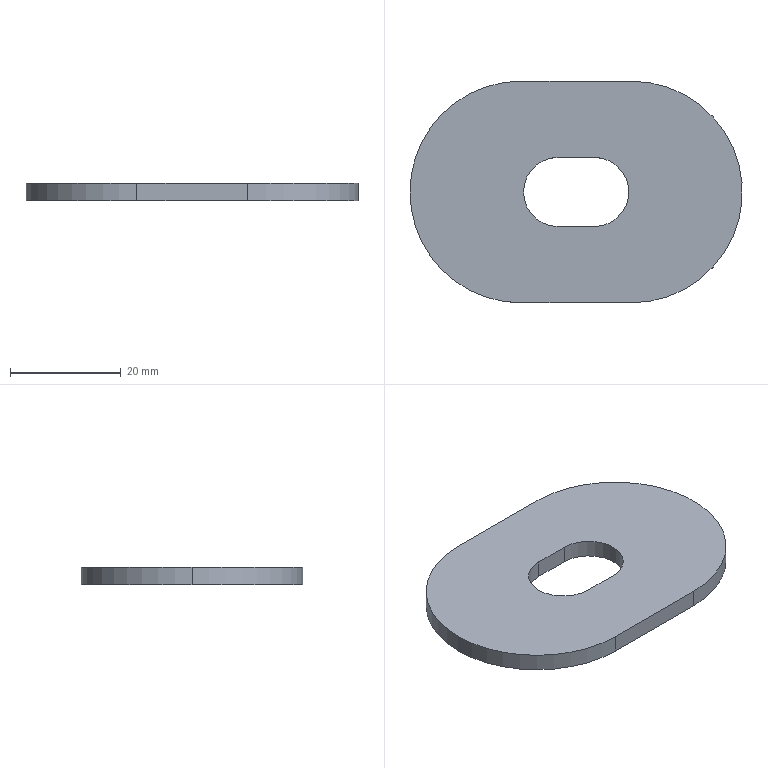Part | SolidWorks | features FlatPattern 1, SMBaseFlange 1, SheetMetal 1 | 1 solid | 12 faces | box 60 x 40 x 3.2 mm | volume 5929 mm3 | cylinder 6 | plane 6 | commonest cylinder face diameters 12.5 x3 40 x3
STEP:
#1=CARTESIAN_POINT('',(575.75,726.25,3.2));
#2=VERTEX_POINT('',#1);
#3=CARTESIAN_POINT('',(569.5,720.,3.2));
#4=VERTEX_POINT('',#3);
#5=CARTESIAN_POINT('',(575.75,720.,3.2));
#6=DIRECTION('',(0.,0.,1.));
#7=DIRECTION('',(1.,0.,0.));
#8=AXIS2_PLACEMENT_3D('',#5,#6,#7);
#9=CIRCLE('',#8,6.25);
#10=EDGE_CURVE('',#2,#4,#9,.T.);
#11=ORIENTED_EDGE('',*,*,#10,.T.);
#12=CARTESIAN_POINT('',(569.5,720.,0.));
#13=VERTEX_POINT('',#12);
#14=CARTESIAN_POINT('',(569.5,720.,3.2));
#15=DIRECTION('',(0.,0.,-1.));
#16=VECTOR('',#15,1000.);
#17=LINE('',#14,#16);
#18=EDGE_CURVE('',#4,#13,#17,.T.);
#19=ORIENTED_EDGE('',*,*,#18,.T.);
#20=CARTESIAN_POINT('',(575.75,726.25,0.));
#21=VERTEX_POINT('',#20);
#22=CARTESIAN_POINT('',(575.75,720.,0.));
#23=DIRECTION('',(0.,0.,1.));
#24=DIRECTION('',(1.,0.,0.));
#25=AXIS2_PLACEMENT_3D('',#22,#23,#24);
#26=CIRCLE('',#25,6.25);
#27=EDGE_CURVE('',#21,#13,#26,.T.);
#28=ORIENTED_EDGE('',*,*,#27,.F.);
#29=CARTESIAN_POINT('',(575.75,726.25,3.2));
#30=DIRECTION('',(0.,0.,-1.));
#31=VECTOR('',#30,1000.);
#32=LINE('',#29,#31);
#33=EDGE_CURVE('',#2,#21,#32,.T.);
#34=ORIENTED_EDGE('',*,*,#33,.F.);
#35=EDGE_LOOP('',(#11,#19,#28,#34));
#36=FACE_OUTER_BOUND('',#35,.T.);
#37=CARTESIAN_POINT('',(575.75,720.,3.2));
#38=DIRECTION('',(0.,0.,-1.));
#39=DIRECTION('',(-1.,0.,0.));
#40=AXIS2_PLACEMENT_3D('',#37,#38,#39);
#41=CYLINDRICAL_SURFACE('',#40,6.25);
#42=ADVANCED_FACE('',(#36),#41,.F.);
#43=CARTESIAN_POINT('',(549.,720.,3.2));
#44=VERTEX_POINT('',#43);
#45=CARTESIAN_POINT('',(569.,700.,3.2));
#46=VERTEX_POINT('',#45);
#47=CARTESIAN_POINT('',(569.,720.,3.2));
#48=DIRECTION('',(0.,0.,1.));
#49=DIRECTION('',(1.,0.,0.));
#50=AXIS2_PLACEMENT_3D('',#47,#48,#49);
#51=CIRCLE('',#50,20.);
#52=EDGE_CURVE('',#44,#46,#51,.T.);
#53=ORIENTED_EDGE('',*,*,#52,.F.);
#54=CARTESIAN_POINT('',(549.,720.,0.));
#55=VERTEX_POINT('',#54);
#56=CARTESIAN_POINT('',(549.,720.,3.2));
#57=DIRECTION('',(0.,0.,-1.));
#58=VECTOR('',#57,1000.);
#59=LINE('',#56,#58);
#60=EDGE_CURVE('',#44,#55,#59,.T.);
#61=ORIENTED_EDGE('',*,*,#60,.T.);
#62=CARTESIAN_POINT('',(569.,700.,0.));
#63=VERTEX_POINT('',#62);
#64=CARTESIAN_POINT('',(569.,720.,0.));
#65=DIRECTION('',(0.,0.,1.));
#66=DIRECTION('',(1.,0.,0.));
#67=AXIS2_PLACEMENT_3D('',#64,#65,#66);
#68=CIRCLE('',#67,20.);
#69=EDGE_CURVE('',#55,#63,#68,.T.);
#70=ORIENTED_EDGE('',*,*,#69,.T.);
#71=CARTESIAN_POINT('',(569.,700.,3.2));
#72=DIRECTION('',(0.,0.,-1.));
#73=VECTOR('',#72,1000.);
#74=LINE('',#71,#73);
#75=EDGE_CURVE('',#46,#63,#74,.T.);
#76=ORIENTED_EDGE('',*,*,#75,.F.);
#77=EDGE_LOOP('',(#53,#61,#70,#76));
#78=FACE_OUTER_BOUND('',#77,.T.);
#79=CARTESIAN_POINT('',(569.,720.,3.2));
#80=DIRECTION('',(0.,0.,-1.));
#81=DIRECTION('',(-1.,0.,0.));
#82=AXIS2_PLACEMENT_3D('',#79,#80,#81);
#83=CYLINDRICAL_SURFACE('',#82,20.);
#84=ADVANCED_FACE('',(#78),#83,.T.);
#85=CARTESIAN_POINT('',(569.,740.,3.2));
#86=VERTEX_POINT('',#85);
#87=CARTESIAN_POINT('',(569.,720.,3.2));
#88=DIRECTION('',(0.,0.,1.));
#89=DIRECTION('',(1.,0.,0.));
#90=AXIS2_PLACEMENT_3D('',#87,#88,#89);
#91=CIRCLE('',#90,20.);
#92=EDGE_CURVE('',#86,#44,#91,.T.);
#93=ORIENTED_EDGE('',*,*,#92,.T.);
#94=ORIENTED_EDGE('',*,*,#52,.T.);
#95=CARTESIAN_POINT('',(589.,700.,3.2));
#96=VERTEX_POINT('',#95);
#97=CARTESIAN_POINT('',(569.,700.,3.2));
#98=DIRECTION('',(1.,0.,0.));
#99=VECTOR('',#98,1000.);
#100=LINE('',#97,#99);
#101=EDGE_CURVE('',#46,#96,#100,.T.);
#102=ORIENTED_EDGE('',*,*,#101,.T.);
#103=CARTESIAN_POINT('',(589.,740.,3.2));
#104=VERTEX_POINT('',#103);
#105=CARTESIAN_POINT('',(589.,720.,3.2));
#106=DIRECTION('',(0.,0.,1.));
#107=DIRECTION('',(1.,0.,0.));
#108=AXIS2_PLACEMENT_3D('',#105,#106,#107);
#109=CIRCLE('',#108,20.);
#110=EDGE_CURVE('',#96,#104,#109,.T.);
#111=ORIENTED_EDGE('',*,*,#110,.T.);
#112=CARTESIAN_POINT('',(569.,740.,3.2));
#113=DIRECTION('',(-1.,0.,0.));
#114=VECTOR('',#113,1000.);
#115=LINE('',#112,#114);
#116=EDGE_CURVE('',#104,#86,#115,.T.);
#117=ORIENTED_EDGE('',*,*,#116,.T.);
#118=EDGE_LOOP('',(#93,#94,#102,#111,#117));
#119=FACE_OUTER_BOUND('',#118,.T.);
#120=CARTESIAN_POINT('',(575.75,713.75,3.2));
#121=VERTEX_POINT('',#120);
#122=CARTESIAN_POINT('',(582.25,713.75,3.2));
#123=VERTEX_POINT('',#122);
#124=CARTESIAN_POINT('',(575.75,713.75,3.2));
#125=DIRECTION('',(1.,0.,0.));
#126=VECTOR('',#125,1000.);
#127=LINE('',#124,#126);
#128=EDGE_CURVE('',#121,#123,#127,.T.);
#129=ORIENTED_EDGE('',*,*,#128,.F.);
#130=CARTESIAN_POINT('',(575.75,720.,3.2));
#131=DIRECTION('',(0.,0.,1.));
#132=DIRECTION('',(1.,0.,0.));
#133=AXIS2_PLACEMENT_3D('',#130,#131,#132);
#134=CIRCLE('',#133,6.25);
#135=EDGE_CURVE('',#4,#121,#134,.T.);
#136=ORIENTED_EDGE('',*,*,#135,.F.);
#137=ORIENTED_EDGE('',*,*,#10,.F.);
#138=CARTESIAN_POINT('',(582.25,726.25,3.2));
#139=VERTEX_POINT('',#138);
#140=CARTESIAN_POINT('',(575.75,726.25,3.2));
#141=DIRECTION('',(-1.,0.,0.));
#142=VECTOR('',#141,1000.);
#143=LINE('',#140,#142);
#144=EDGE_CURVE('',#139,#2,#143,.T.);
#145=ORIENTED_EDGE('',*,*,#144,.F.);
#146=CARTESIAN_POINT('',(582.25,720.,3.2));
#147=DIRECTION('',(0.,0.,1.));
#148=DIRECTION('',(1.,0.,0.));
#149=AXIS2_PLACEMENT_3D('',#146,#147,#148);
#150=CIRCLE('',#149,6.25);
#151=EDGE_CURVE('',#123,#139,#150,.T.);
#152=ORIENTED_EDGE('',*,*,#151,.F.);
#153=EDGE_LOOP('',(#129,#136,#137,#145,#152));
#154=FACE_BOUND('',#153,.T.);
#155=CARTESIAN_POINT('',(569.,720.,3.2));
#156=DIRECTION('',(0.,0.,1.));
#157=DIRECTION('',(1.,0.,0.));
#158=AXIS2_PLACEMENT_3D('',#155,#156,#157);
#159=PLANE('',#158);
#160=ADVANCED_FACE('',(#119,#154),#159,.T.);
#161=CARTESIAN_POINT('',(569.,740.,0.));
#162=VERTEX_POINT('',#161);
#163=CARTESIAN_POINT('',(569.,720.,0.));
#164=DIRECTION('',(0.,0.,1.));
#165=DIRECTION('',(1.,0.,0.));
#166=AXIS2_PLACEMENT_3D('',#163,#164,#165);
#167=CIRCLE('',#166,20.);
#168=EDGE_CURVE('',#162,#55,#167,.T.);
#169=ORIENTED_EDGE('',*,*,#168,.F.);
#170=CARTESIAN_POINT('',(589.,740.,0.));
#171=VERTEX_POINT('',#170);
#172=CARTESIAN_POINT('',(569.,740.,0.));
#173=DIRECTION('',(-1.,0.,0.));
#174=VECTOR('',#173,1000.);
#175=LINE('',#172,#174);
#176=EDGE_CURVE('',#171,#162,#175,.T.);
#177=ORIENTED_EDGE('',*,*,#176,.F.);
#178=CARTESIAN_POINT('',(589.,700.,0.));
#179=VERTEX_POINT('',#178);
#180=CARTESIAN_POINT('',(589.,720.,0.));
#181=DIRECTION('',(0.,0.,1.));
#182=DIRECTION('',(1.,0.,0.));
#183=AXIS2_PLACEMENT_3D('',#180,#181,#182);
#184=CIRCLE('',#183,20.);
#185=EDGE_CURVE('',#179,#171,#184,.T.);
#186=ORIENTED_EDGE('',*,*,#185,.F.);
#187=CARTESIAN_POINT('',(569.,700.,0.));
#188=DIRECTION('',(1.,0.,0.));
#189=VECTOR('',#188,1000.);
#190=LINE('',#187,#189);
#191=EDGE_CURVE('',#63,#179,#190,.T.);
#192=ORIENTED_EDGE('',*,*,#191,.F.);
#193=ORIENTED_EDGE('',*,*,#69,.F.);
#194=EDGE_LOOP('',(#169,#177,#186,#192,#193));
#195=FACE_OUTER_BOUND('',#194,.T.);
#196=ORIENTED_EDGE('',*,*,#27,.T.);
#197=CARTESIAN_POINT('',(575.75,713.75,0.));
#198=VERTEX_POINT('',#197);
#199=CARTESIAN_POINT('',(575.75,720.,0.));
#200=DIRECTION('',(0.,0.,1.));
#201=DIRECTION('',(1.,0.,0.));
#202=AXIS2_PLACEMENT_3D('',#199,#200,#201);
#203=CIRCLE('',#202,6.25);
#204=EDGE_CURVE('',#13,#198,#203,.T.);
#205=ORIENTED_EDGE('',*,*,#204,.T.);
#206=CARTESIAN_POINT('',(582.25,713.75,0.));
#207=VERTEX_POINT('',#206);
#208=CARTESIAN_POINT('',(575.75,713.75,0.));
#209=DIRECTION('',(1.,0.,0.));
#210=VECTOR('',#209,1000.);
#211=LINE('',#208,#210);
#212=EDGE_CURVE('',#198,#207,#211,.T.);
#213=ORIENTED_EDGE('',*,*,#212,.T.);
#214=CARTESIAN_POINT('',(582.25,726.25,0.));
#215=VERTEX_POINT('',#214);
#216=CARTESIAN_POINT('',(582.25,720.,0.));
#217=DIRECTION('',(0.,0.,1.));
#218=DIRECTION('',(1.,0.,0.));
#219=AXIS2_PLACEMENT_3D('',#216,#217,#218);
#220=CIRCLE('',#219,6.25);
#221=EDGE_CURVE('',#207,#215,#220,.T.);
#222=ORIENTED_EDGE('',*,*,#221,.T.);
#223=CARTESIAN_POINT('',(575.75,726.25,0.));
#224=DIRECTION('',(-1.,0.,0.));
#225=VECTOR('',#224,1000.);
#226=LINE('',#223,#225);
#227=EDGE_CURVE('',#215,#21,#226,.T.);
#228=ORIENTED_EDGE('',*,*,#227,.T.);
#229=EDGE_LOOP('',(#196,#205,#213,#222,#228));
#230=FACE_BOUND('',#229,.T.);
#231=CARTESIAN_POINT('',(569.,720.,0.));
#232=DIRECTION('',(0.,0.,1.));
#233=DIRECTION('',(1.,0.,0.));
#234=AXIS2_PLACEMENT_3D('',#231,#232,#233);
#235=PLANE('',#234);
#236=ADVANCED_FACE('',(#195,#230),#235,.F.);
#237=ORIENTED_EDGE('',*,*,#60,.F.);
#238=ORIENTED_EDGE('',*,*,#92,.F.);
#239=CARTESIAN_POINT('',(569.,740.,3.2));
#240=DIRECTION('',(0.,0.,-1.));
#241=VECTOR('',#240,1000.);
#242=LINE('',#239,#241);
#243=EDGE_CURVE('',#86,#162,#242,.T.);
#244=ORIENTED_EDGE('',*,*,#243,.T.);
#245=ORIENTED_EDGE('',*,*,#168,.T.);
#246=EDGE_LOOP('',(#237,#238,#244,#245));
#247=FACE_OUTER_BOUND('',#246,.T.);
#248=CARTESIAN_POINT('',(569.,720.,3.2));
#249=DIRECTION('',(0.,0.,-1.));
#250=DIRECTION('',(-1.,0.,0.));
#251=AXIS2_PLACEMENT_3D('',#248,#249,#250);
#252=CYLINDRICAL_SURFACE('',#251,20.);
#253=ADVANCED_FACE('',(#247),#252,.T.);
#254=ORIENTED_EDGE('',*,*,#191,.T.);
#255=CARTESIAN_POINT('',(589.,700.,3.2));
#256=DIRECTION('',(0.,0.,-1.));
#257=VECTOR('',#256,1000.);
#258=LINE('',#255,#257);
#259=EDGE_CURVE('',#96,#179,#258,.T.);
#260=ORIENTED_EDGE('',*,*,#259,.F.);
#261=ORIENTED_EDGE('',*,*,#101,.F.);
#262=ORIENTED_EDGE('',*,*,#75,.T.);
#263=EDGE_LOOP('',(#254,#260,#261,#262));
#264=FACE_OUTER_BOUND('',#263,.T.);
#265=CARTESIAN_POINT('',(569.,700.,3.2));
#266=DIRECTION('',(0.,1.,0.));
#267=DIRECTION('',(0.,0.,1.));
#268=AXIS2_PLACEMENT_3D('',#265,#266,#267);
#269=PLANE('',#268);
#270=ADVANCED_FACE('',(#264),#269,.F.);
#271=ORIENTED_EDGE('',*,*,#185,.T.);
#272=CARTESIAN_POINT('',(589.,740.,3.2));
#273=DIRECTION('',(0.,0.,-1.));
#274=VECTOR('',#273,1000.);
#275=LINE('',#272,#274);
#276=EDGE_CURVE('',#104,#171,#275,.T.);
#277=ORIENTED_EDGE('',*,*,#276,.F.);
#278=ORIENTED_EDGE('',*,*,#110,.F.);
#279=ORIENTED_EDGE('',*,*,#259,.T.);
#280=EDGE_LOOP('',(#271,#277,#278,#279));
#281=FACE_OUTER_BOUND('',#280,.T.);
#282=CARTESIAN_POINT('',(589.,720.,3.2));
#283=DIRECTION('',(0.,0.,-1.));
#284=DIRECTION('',(-1.,0.,0.));
#285=AXIS2_PLACEMENT_3D('',#282,#283,#284);
#286=CYLINDRICAL_SURFACE('',#285,20.);
#287=ADVANCED_FACE('',(#281),#286,.T.);
#288=ORIENTED_EDGE('',*,*,#176,.T.);
#289=ORIENTED_EDGE('',*,*,#243,.F.);
#290=ORIENTED_EDGE('',*,*,#116,.F.);
#291=ORIENTED_EDGE('',*,*,#276,.T.);
#292=EDGE_LOOP('',(#288,#289,#290,#291));
#293=FACE_OUTER_BOUND('',#292,.T.);
#294=CARTESIAN_POINT('',(569.,740.,3.2));
#295=DIRECTION('',(0.,-1.,0.));
#296=DIRECTION('',(0.,0.,-1.));
#297=AXIS2_PLACEMENT_3D('',#294,#295,#296);
#298=PLANE('',#297);
#299=ADVANCED_FACE('',(#293),#298,.F.);
#300=ORIENTED_EDGE('',*,*,#18,.F.);
#301=ORIENTED_EDGE('',*,*,#135,.T.);
#302=CARTESIAN_POINT('',(575.75,713.75,3.2));
#303=DIRECTION('',(0.,0.,-1.));
#304=VECTOR('',#303,1000.);
#305=LINE('',#302,#304);
#306=EDGE_CURVE('',#121,#198,#305,.T.);
#307=ORIENTED_EDGE('',*,*,#306,.T.);
#308=ORIENTED_EDGE('',*,*,#204,.F.);
#309=EDGE_LOOP('',(#300,#301,#307,#308));
#310=FACE_OUTER_BOUND('',#309,.T.);
#311=CARTESIAN_POINT('',(575.75,720.,3.2));
#312=DIRECTION('',(0.,0.,-1.));
#313=DIRECTION('',(-1.,0.,0.));
#314=AXIS2_PLACEMENT_3D('',#311,#312,#313);
#315=CYLINDRICAL_SURFACE('',#314,6.25);
#316=ADVANCED_FACE('',(#310),#315,.F.);
#317=ORIENTED_EDGE('',*,*,#212,.F.);
#318=ORIENTED_EDGE('',*,*,#306,.F.);
#319=ORIENTED_EDGE('',*,*,#128,.T.);
#320=CARTESIAN_POINT('',(582.25,713.75,3.2));
#321=DIRECTION('',(0.,0.,-1.));
#322=VECTOR('',#321,1000.);
#323=LINE('',#320,#322);
#324=EDGE_CURVE('',#123,#207,#323,.T.);
#325=ORIENTED_EDGE('',*,*,#324,.T.);
#326=EDGE_LOOP('',(#317,#318,#319,#325));
#327=FACE_OUTER_BOUND('',#326,.T.);
#328=CARTESIAN_POINT('',(575.75,713.75,3.2));
#329=DIRECTION('',(0.,1.,0.));
#330=DIRECTION('',(0.,0.,1.));
#331=AXIS2_PLACEMENT_3D('',#328,#329,#330);
#332=PLANE('',#331);
#333=ADVANCED_FACE('',(#327),#332,.T.);
#334=ORIENTED_EDGE('',*,*,#221,.F.);
#335=ORIENTED_EDGE('',*,*,#324,.F.);
#336=ORIENTED_EDGE('',*,*,#151,.T.);
#337=CARTESIAN_POINT('',(582.25,726.25,3.2));
#338=DIRECTION('',(0.,0.,-1.));
#339=VECTOR('',#338,1000.);
#340=LINE('',#337,#339);
#341=EDGE_CURVE('',#139,#215,#340,.T.);
#342=ORIENTED_EDGE('',*,*,#341,.T.);
#343=EDGE_LOOP('',(#334,#335,#336,#342));
#344=FACE_OUTER_BOUND('',#343,.T.);
#345=CARTESIAN_POINT('',(582.25,720.,3.2));
#346=DIRECTION('',(0.,0.,-1.));
#347=DIRECTION('',(-1.,0.,0.));
#348=AXIS2_PLACEMENT_3D('',#345,#346,#347);
#349=CYLINDRICAL_SURFACE('',#348,6.25);
#350=ADVANCED_FACE('',(#344),#349,.F.);
#351=ORIENTED_EDGE('',*,*,#227,.F.);
#352=ORIENTED_EDGE('',*,*,#341,.F.);
#353=ORIENTED_EDGE('',*,*,#144,.T.);
#354=ORIENTED_EDGE('',*,*,#33,.T.);
#355=EDGE_LOOP('',(#351,#352,#353,#354));
#356=FACE_OUTER_BOUND('',#355,.T.);
#357=CARTESIAN_POINT('',(575.75,726.25,3.2));
#358=DIRECTION('',(0.,-1.,0.));
#359=DIRECTION('',(0.,0.,-1.));
#360=AXIS2_PLACEMENT_3D('',#357,#358,#359);
#361=PLANE('',#360);
#362=ADVANCED_FACE('',(#356),#361,.T.);
#363=CLOSED_SHELL('',(#42,#84,#160,#236,#253,#270,#287,#299,#316,#333,#350,#362));
#364=MANIFOLD_SOLID_BREP('',#363);
#365=CARTESIAN_POINT('',(0.,0.,0.));
#366=DIRECTION('',(0.,0.,1.));
#367=DIRECTION('',(1.,0.,0.));
#368=AXIS2_PLACEMENT_3D('',#365,#366,#367);
#369=(LENGTH_UNIT()NAMED_UNIT(*)SI_UNIT(.MILLI.,.METRE.));
#370=UNCERTAINTY_MEASURE_WITH_UNIT(LENGTH_MEASURE(0.00001),#369,'','');
#371=(NAMED_UNIT(*)PLANE_ANGLE_UNIT()SI_UNIT($,.RADIAN.));
#372=(NAMED_UNIT(*)SI_UNIT($,.STERADIAN.)SOLID_ANGLE_UNIT());
#373=(GEOMETRIC_REPRESENTATION_CONTEXT(3)GLOBAL_UNCERTAINTY_ASSIGNED_CONTEXT((#370))GLOBAL_UNIT_ASSIGNED_CONTEXT((#369,#371,#372))REPRESENTATION_CONTEXT('',''));
#374=ADVANCED_BREP_SHAPE_REPRESENTATION('',(#364,#368),#373);